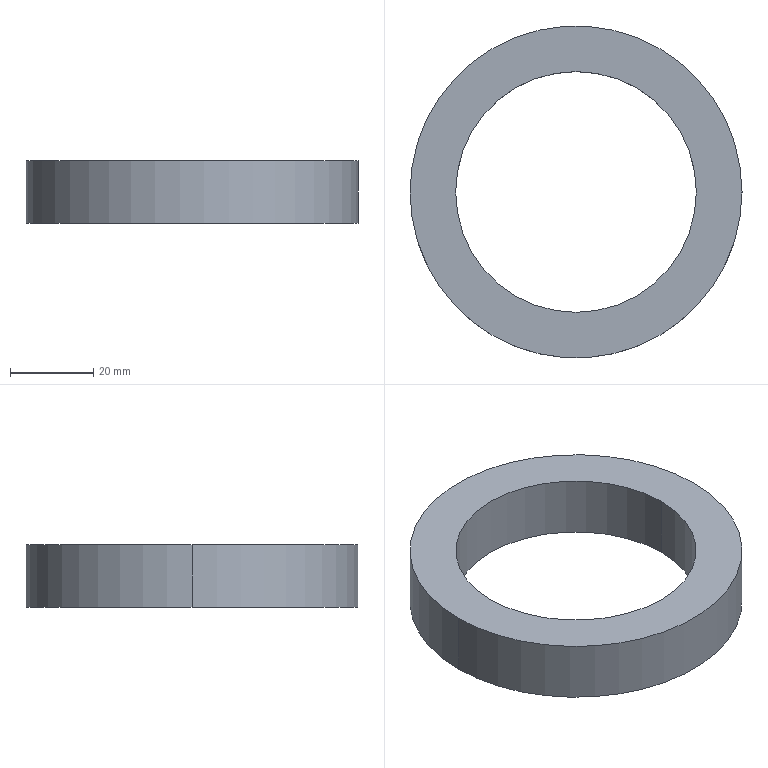Part | SolidWorks | features BaseBody 1 | 1 solid | 6 faces | box 80 x 80 x 15 mm | volume 35767 mm3 | cylinder 4 | plane 2 | commonest cylinder face diameters 58 x2 80 x2
STEP:
#1=CARTESIAN_POINT('',(29.,0.,15.));
#2=VERTEX_POINT('',#1);
#3=CARTESIAN_POINT('',(-29.,0.,15.));
#4=VERTEX_POINT('',#3);
#5=CARTESIAN_POINT('',(0.,0.,15.));
#6=DIRECTION('',(0.,0.,-1.));
#7=DIRECTION('',(-1.,0.,0.));
#8=AXIS2_PLACEMENT_3D('',#5,#6,#7);
#9=CIRCLE('',#8,29.);
#10=EDGE_CURVE('',#2,#4,#9,.T.);
#11=ORIENTED_EDGE('',*,*,#10,.F.);
#12=CARTESIAN_POINT('',(29.,0.,0.));
#13=VERTEX_POINT('',#12);
#14=CARTESIAN_POINT('',(29.,0.,15.));
#15=DIRECTION('',(0.,0.,-1.));
#16=VECTOR('',#15,1000.);
#17=LINE('',#14,#16);
#18=EDGE_CURVE('',#2,#13,#17,.T.);
#19=ORIENTED_EDGE('',*,*,#18,.T.);
#20=CARTESIAN_POINT('',(-29.,0.,0.));
#21=VERTEX_POINT('',#20);
#22=CARTESIAN_POINT('',(0.,0.,0.));
#23=DIRECTION('',(0.,0.,1.));
#24=DIRECTION('',(-1.,0.,0.));
#25=AXIS2_PLACEMENT_3D('',#22,#23,#24);
#26=CIRCLE('',#25,29.);
#27=EDGE_CURVE('',#21,#13,#26,.T.);
#28=ORIENTED_EDGE('',*,*,#27,.F.);
#29=CARTESIAN_POINT('',(-29.,0.,15.));
#30=DIRECTION('',(0.,0.,-1.));
#31=VECTOR('',#30,1000.);
#32=LINE('',#29,#31);
#33=EDGE_CURVE('',#4,#21,#32,.T.);
#34=ORIENTED_EDGE('',*,*,#33,.F.);
#35=EDGE_LOOP('',(#11,#19,#28,#34));
#36=FACE_OUTER_BOUND('',#35,.T.);
#37=CARTESIAN_POINT('',(0.,0.,15.));
#38=DIRECTION('',(0.,0.,-1.));
#39=DIRECTION('',(-1.,0.,0.));
#40=AXIS2_PLACEMENT_3D('',#37,#38,#39);
#41=CYLINDRICAL_SURFACE('',#40,29.);
#42=ADVANCED_FACE('',(#36),#41,.F.);
#43=CARTESIAN_POINT('',(40.,0.,15.));
#44=VERTEX_POINT('',#43);
#45=CARTESIAN_POINT('',(-40.,0.,15.));
#46=VERTEX_POINT('',#45);
#47=CARTESIAN_POINT('',(0.,0.,15.));
#48=DIRECTION('',(0.,0.,1.));
#49=DIRECTION('',(-1.,0.,0.));
#50=AXIS2_PLACEMENT_3D('',#47,#48,#49);
#51=CIRCLE('',#50,40.);
#52=EDGE_CURVE('',#44,#46,#51,.T.);
#53=ORIENTED_EDGE('',*,*,#52,.F.);
#54=CARTESIAN_POINT('',(40.,0.,0.));
#55=VERTEX_POINT('',#54);
#56=CARTESIAN_POINT('',(40.,0.,15.));
#57=DIRECTION('',(0.,0.,-1.));
#58=VECTOR('',#57,1000.);
#59=LINE('',#56,#58);
#60=EDGE_CURVE('',#44,#55,#59,.T.);
#61=ORIENTED_EDGE('',*,*,#60,.T.);
#62=CARTESIAN_POINT('',(-40.,0.,0.));
#63=VERTEX_POINT('',#62);
#64=CARTESIAN_POINT('',(0.,0.,0.));
#65=DIRECTION('',(0.,0.,1.));
#66=DIRECTION('',(-1.,0.,0.));
#67=AXIS2_PLACEMENT_3D('',#64,#65,#66);
#68=CIRCLE('',#67,40.);
#69=EDGE_CURVE('',#55,#63,#68,.T.);
#70=ORIENTED_EDGE('',*,*,#69,.T.);
#71=CARTESIAN_POINT('',(-40.,0.,15.));
#72=DIRECTION('',(0.,0.,-1.));
#73=VECTOR('',#72,1000.);
#74=LINE('',#71,#73);
#75=EDGE_CURVE('',#46,#63,#74,.T.);
#76=ORIENTED_EDGE('',*,*,#75,.F.);
#77=EDGE_LOOP('',(#53,#61,#70,#76));
#78=FACE_OUTER_BOUND('',#77,.T.);
#79=CARTESIAN_POINT('',(0.,0.,15.));
#80=DIRECTION('',(0.,0.,-1.));
#81=DIRECTION('',(-1.,0.,0.));
#82=AXIS2_PLACEMENT_3D('',#79,#80,#81);
#83=CYLINDRICAL_SURFACE('',#82,40.);
#84=ADVANCED_FACE('',(#78),#83,.T.);
#85=CARTESIAN_POINT('',(0.,0.,15.));
#86=DIRECTION('',(0.,0.,-1.));
#87=DIRECTION('',(-1.,0.,0.));
#88=AXIS2_PLACEMENT_3D('',#85,#86,#87);
#89=CIRCLE('',#88,29.);
#90=EDGE_CURVE('',#4,#2,#89,.T.);
#91=ORIENTED_EDGE('',*,*,#90,.T.);
#92=ORIENTED_EDGE('',*,*,#10,.T.);
#93=EDGE_LOOP('',(#91,#92));
#94=FACE_BOUND('',#93,.T.);
#95=CARTESIAN_POINT('',(0.,0.,15.));
#96=DIRECTION('',(0.,0.,1.));
#97=DIRECTION('',(-1.,0.,0.));
#98=AXIS2_PLACEMENT_3D('',#95,#96,#97);
#99=CIRCLE('',#98,40.);
#100=EDGE_CURVE('',#46,#44,#99,.T.);
#101=ORIENTED_EDGE('',*,*,#100,.T.);
#102=ORIENTED_EDGE('',*,*,#52,.T.);
#103=EDGE_LOOP('',(#101,#102));
#104=FACE_OUTER_BOUND('',#103,.T.);
#105=CARTESIAN_POINT('',(0.,0.,15.));
#106=DIRECTION('',(0.,0.,1.));
#107=DIRECTION('',(1.,0.,0.));
#108=AXIS2_PLACEMENT_3D('',#105,#106,#107);
#109=PLANE('',#108);
#110=ADVANCED_FACE('',(#94,#104),#109,.T.);
#111=ORIENTED_EDGE('',*,*,#18,.F.);
#112=ORIENTED_EDGE('',*,*,#90,.F.);
#113=ORIENTED_EDGE('',*,*,#33,.T.);
#114=CARTESIAN_POINT('',(0.,0.,0.));
#115=DIRECTION('',(0.,0.,1.));
#116=DIRECTION('',(-1.,0.,0.));
#117=AXIS2_PLACEMENT_3D('',#114,#115,#116);
#118=CIRCLE('',#117,29.);
#119=EDGE_CURVE('',#13,#21,#118,.T.);
#120=ORIENTED_EDGE('',*,*,#119,.F.);
#121=EDGE_LOOP('',(#111,#112,#113,#120));
#122=FACE_OUTER_BOUND('',#121,.T.);
#123=CARTESIAN_POINT('',(0.,0.,15.));
#124=DIRECTION('',(0.,0.,-1.));
#125=DIRECTION('',(-1.,0.,0.));
#126=AXIS2_PLACEMENT_3D('',#123,#124,#125);
#127=CYLINDRICAL_SURFACE('',#126,29.);
#128=ADVANCED_FACE('',(#122),#127,.F.);
#129=ORIENTED_EDGE('',*,*,#60,.F.);
#130=ORIENTED_EDGE('',*,*,#100,.F.);
#131=ORIENTED_EDGE('',*,*,#75,.T.);
#132=CARTESIAN_POINT('',(0.,0.,0.));
#133=DIRECTION('',(0.,0.,1.));
#134=DIRECTION('',(-1.,0.,0.));
#135=AXIS2_PLACEMENT_3D('',#132,#133,#134);
#136=CIRCLE('',#135,40.);
#137=EDGE_CURVE('',#63,#55,#136,.T.);
#138=ORIENTED_EDGE('',*,*,#137,.T.);
#139=EDGE_LOOP('',(#129,#130,#131,#138));
#140=FACE_OUTER_BOUND('',#139,.T.);
#141=CARTESIAN_POINT('',(0.,0.,15.));
#142=DIRECTION('',(0.,0.,-1.));
#143=DIRECTION('',(-1.,0.,0.));
#144=AXIS2_PLACEMENT_3D('',#141,#142,#143);
#145=CYLINDRICAL_SURFACE('',#144,40.);
#146=ADVANCED_FACE('',(#140),#145,.T.);
#147=ORIENTED_EDGE('',*,*,#27,.T.);
#148=ORIENTED_EDGE('',*,*,#119,.T.);
#149=EDGE_LOOP('',(#147,#148));
#150=FACE_BOUND('',#149,.T.);
#151=ORIENTED_EDGE('',*,*,#137,.F.);
#152=ORIENTED_EDGE('',*,*,#69,.F.);
#153=EDGE_LOOP('',(#151,#152));
#154=FACE_OUTER_BOUND('',#153,.T.);
#155=CARTESIAN_POINT('',(0.,0.,0.));
#156=DIRECTION('',(0.,0.,1.));
#157=DIRECTION('',(1.,0.,0.));
#158=AXIS2_PLACEMENT_3D('',#155,#156,#157);
#159=PLANE('',#158);
#160=ADVANCED_FACE('',(#150,#154),#159,.F.);
#161=CLOSED_SHELL('',(#42,#84,#110,#128,#146,#160));
#162=MANIFOLD_SOLID_BREP('',#161);
#163=CARTESIAN_POINT('',(0.,0.,0.));
#164=DIRECTION('',(0.,0.,1.));
#165=DIRECTION('',(1.,0.,0.));
#166=AXIS2_PLACEMENT_3D('',#163,#164,#165);
#167=(LENGTH_UNIT()NAMED_UNIT(*)SI_UNIT(.MILLI.,.METRE.));
#168=UNCERTAINTY_MEASURE_WITH_UNIT(LENGTH_MEASURE(0.00001),#167,'','');
#169=(NAMED_UNIT(*)PLANE_ANGLE_UNIT()SI_UNIT($,.RADIAN.));
#170=(NAMED_UNIT(*)SI_UNIT($,.STERADIAN.)SOLID_ANGLE_UNIT());
#171=(GEOMETRIC_REPRESENTATION_CONTEXT(3)GLOBAL_UNCERTAINTY_ASSIGNED_CONTEXT((#168))GLOBAL_UNIT_ASSIGNED_CONTEXT((#167,#169,#170))REPRESENTATION_CONTEXT('',''));
#172=ADVANCED_BREP_SHAPE_REPRESENTATION('',(#162,#166),#171);